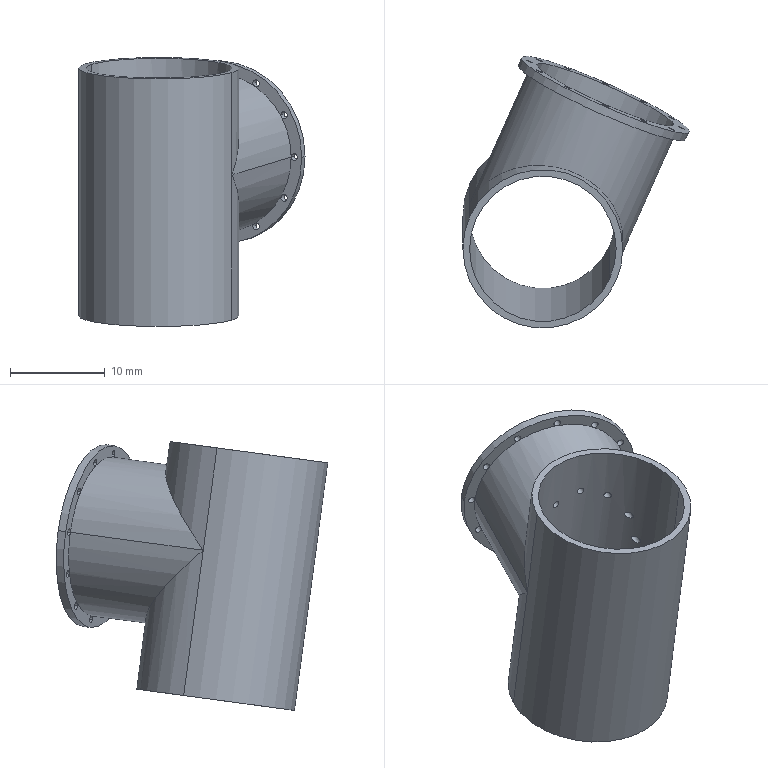Part | SolidWorks | features SplitBody 1 | 1 solid | 94 faces | box 23.905 x 28.753 x 28.421 mm | volume 2021 mm3 | cylinder 68 | plane 26 | commonest cylinder face diameters 0.739 x48 16.896 x5 3.52 x3 2.464 x2 8.096 x2 14.784 x2